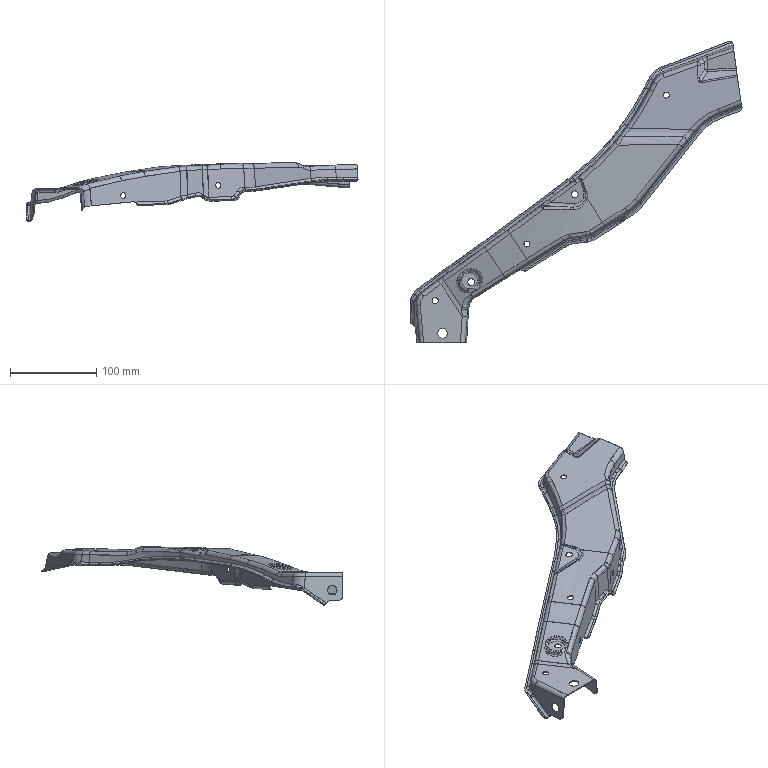Part | 1 solid | 461 faces | box 385.938 x 350.086 x 68.276 mm | volume 60277 mm3 | spline 297 | cylinder 121 | plane 36 | other 5 | sphere 2 | commonest cylinder face diameters 6 x14 8.4 x14 8 x10 11 x10 10 x9 5.6 x6